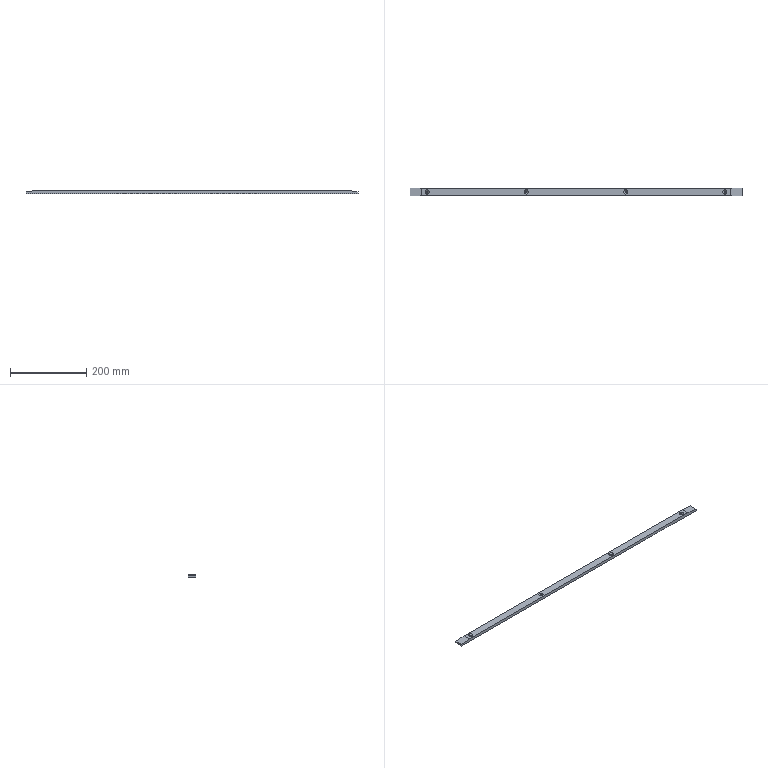Part | SolidWorks | features BaseBody 1 | 1 solid | 24 faces | box 870 x 20 x 8 mm | volume 136262 mm3 | cone 8 | cylinder 8 | plane 8 | commonest cylinder face diameters 5.5 x8
STEP:
#1=CARTESIAN_POINT('',(-392.75,0.,5.15));
#2=VERTEX_POINT('',#1);
#3=CARTESIAN_POINT('',(-387.25,0.,5.15));
#4=VERTEX_POINT('',#3);
#5=CARTESIAN_POINT('',(-390.,0.,5.15));
#6=DIRECTION('',(0.,0.,1.));
#7=DIRECTION('',(1.,0.,0.));
#8=AXIS2_PLACEMENT_3D('',#5,#6,#7);
#9=CIRCLE('',#8,2.75);
#10=EDGE_CURVE('',#2,#4,#9,.T.);
#11=ORIENTED_EDGE('',*,*,#10,.F.);
#12=CARTESIAN_POINT('',(-395.6,0.,8.));
#13=VERTEX_POINT('',#12);
#14=CARTESIAN_POINT('',(-395.6,0.,8.));
#15=DIRECTION('',(-0.7071,0.,0.7071));
#16=VECTOR('',#15,1000.);
#17=LINE('',#14,#16);
#18=EDGE_CURVE('',#2,#13,#17,.T.);
#19=ORIENTED_EDGE('',*,*,#18,.T.);
#20=CARTESIAN_POINT('',(-384.4,0.,8.));
#21=VERTEX_POINT('',#20);
#22=CARTESIAN_POINT('',(-390.,0.,8.));
#23=DIRECTION('',(0.,0.,1.));
#24=DIRECTION('',(1.,0.,0.));
#25=AXIS2_PLACEMENT_3D('',#22,#23,#24);
#26=CIRCLE('',#25,5.6);
#27=EDGE_CURVE('',#13,#21,#26,.T.);
#28=ORIENTED_EDGE('',*,*,#27,.T.);
#29=CARTESIAN_POINT('',(-384.4,0.,8.));
#30=DIRECTION('',(0.7071,0.,0.7071));
#31=VECTOR('',#30,1000.);
#32=LINE('',#29,#31);
#33=EDGE_CURVE('',#4,#21,#32,.T.);
#34=ORIENTED_EDGE('',*,*,#33,.F.);
#35=EDGE_LOOP('',(#11,#19,#28,#34));
#36=FACE_OUTER_BOUND('',#35,.T.);
#37=CARTESIAN_POINT('',(-390.,0.,8.));
#38=DIRECTION('',(0.,0.,1.));
#39=DIRECTION('',(1.,0.,0.));
#40=AXIS2_PLACEMENT_3D('',#37,#38,#39);
#41=CONICAL_SURFACE('',#40,5.6,0.7854);
#42=ADVANCED_FACE('',(#36),#41,.F.);
#43=CARTESIAN_POINT('',(-392.75,0.,0.));
#44=VERTEX_POINT('',#43);
#45=CARTESIAN_POINT('',(-387.25,0.,0.));
#46=VERTEX_POINT('',#45);
#47=CARTESIAN_POINT('',(-390.,0.,0.));
#48=DIRECTION('',(0.,0.,1.));
#49=DIRECTION('',(1.,0.,0.));
#50=AXIS2_PLACEMENT_3D('',#47,#48,#49);
#51=CIRCLE('',#50,2.75);
#52=EDGE_CURVE('',#44,#46,#51,.T.);
#53=ORIENTED_EDGE('',*,*,#52,.F.);
#54=CARTESIAN_POINT('',(-392.75,0.,8.));
#55=DIRECTION('',(0.,0.,1.));
#56=VECTOR('',#55,1000.);
#57=LINE('',#54,#56);
#58=EDGE_CURVE('',#44,#2,#57,.T.);
#59=ORIENTED_EDGE('',*,*,#58,.T.);
#60=ORIENTED_EDGE('',*,*,#10,.T.);
#61=CARTESIAN_POINT('',(-387.25,0.,8.));
#62=DIRECTION('',(0.,0.,1.));
#63=VECTOR('',#62,1000.);
#64=LINE('',#61,#63);
#65=EDGE_CURVE('',#46,#4,#64,.T.);
#66=ORIENTED_EDGE('',*,*,#65,.F.);
#67=EDGE_LOOP('',(#53,#59,#60,#66));
#68=FACE_OUTER_BOUND('',#67,.T.);
#69=CARTESIAN_POINT('',(-390.,0.,8.));
#70=DIRECTION('',(0.,0.,1.));
#71=DIRECTION('',(1.,0.,0.));
#72=AXIS2_PLACEMENT_3D('',#69,#70,#71);
#73=CYLINDRICAL_SURFACE('',#72,2.75);
#74=ADVANCED_FACE('',(#68),#73,.F.);
#75=CARTESIAN_POINT('',(-132.75,0.,5.15));
#76=VERTEX_POINT('',#75);
#77=CARTESIAN_POINT('',(-127.25,0.,5.15));
#78=VERTEX_POINT('',#77);
#79=CARTESIAN_POINT('',(-130.,0.,5.15));
#80=DIRECTION('',(0.,0.,1.));
#81=DIRECTION('',(1.,0.,0.));
#82=AXIS2_PLACEMENT_3D('',#79,#80,#81);
#83=CIRCLE('',#82,2.75);
#84=EDGE_CURVE('',#76,#78,#83,.T.);
#85=ORIENTED_EDGE('',*,*,#84,.F.);
#86=CARTESIAN_POINT('',(-135.6,0.,8.));
#87=VERTEX_POINT('',#86);
#88=CARTESIAN_POINT('',(-135.6,0.,8.));
#89=DIRECTION('',(-0.7071,0.,0.7071));
#90=VECTOR('',#89,1000.);
#91=LINE('',#88,#90);
#92=EDGE_CURVE('',#76,#87,#91,.T.);
#93=ORIENTED_EDGE('',*,*,#92,.T.);
#94=CARTESIAN_POINT('',(-124.4,0.,8.));
#95=VERTEX_POINT('',#94);
#96=CARTESIAN_POINT('',(-130.,0.,8.));
#97=DIRECTION('',(0.,0.,1.));
#98=DIRECTION('',(1.,0.,0.));
#99=AXIS2_PLACEMENT_3D('',#96,#97,#98);
#100=CIRCLE('',#99,5.6);
#101=EDGE_CURVE('',#87,#95,#100,.T.);
#102=ORIENTED_EDGE('',*,*,#101,.T.);
#103=CARTESIAN_POINT('',(-124.4,0.,8.));
#104=DIRECTION('',(0.7071,0.,0.7071));
#105=VECTOR('',#104,1000.);
#106=LINE('',#103,#105);
#107=EDGE_CURVE('',#78,#95,#106,.T.);
#108=ORIENTED_EDGE('',*,*,#107,.F.);
#109=EDGE_LOOP('',(#85,#93,#102,#108));
#110=FACE_OUTER_BOUND('',#109,.T.);
#111=CARTESIAN_POINT('',(-130.,0.,8.));
#112=DIRECTION('',(0.,0.,1.));
#113=DIRECTION('',(1.,0.,0.));
#114=AXIS2_PLACEMENT_3D('',#111,#112,#113);
#115=CONICAL_SURFACE('',#114,5.6,0.7854);
#116=ADVANCED_FACE('',(#110),#115,.F.);
#117=CARTESIAN_POINT('',(-132.75,0.,0.));
#118=VERTEX_POINT('',#117);
#119=CARTESIAN_POINT('',(-127.25,0.,0.));
#120=VERTEX_POINT('',#119);
#121=CARTESIAN_POINT('',(-130.,0.,0.));
#122=DIRECTION('',(0.,0.,1.));
#123=DIRECTION('',(1.,0.,0.));
#124=AXIS2_PLACEMENT_3D('',#121,#122,#123);
#125=CIRCLE('',#124,2.75);
#126=EDGE_CURVE('',#118,#120,#125,.T.);
#127=ORIENTED_EDGE('',*,*,#126,.F.);
#128=CARTESIAN_POINT('',(-132.75,0.,8.));
#129=DIRECTION('',(0.,0.,1.));
#130=VECTOR('',#129,1000.);
#131=LINE('',#128,#130);
#132=EDGE_CURVE('',#118,#76,#131,.T.);
#133=ORIENTED_EDGE('',*,*,#132,.T.);
#134=ORIENTED_EDGE('',*,*,#84,.T.);
#135=CARTESIAN_POINT('',(-127.25,0.,8.));
#136=DIRECTION('',(0.,0.,1.));
#137=VECTOR('',#136,1000.);
#138=LINE('',#135,#137);
#139=EDGE_CURVE('',#120,#78,#138,.T.);
#140=ORIENTED_EDGE('',*,*,#139,.F.);
#141=EDGE_LOOP('',(#127,#133,#134,#140));
#142=FACE_OUTER_BOUND('',#141,.T.);
#143=CARTESIAN_POINT('',(-130.,0.,8.));
#144=DIRECTION('',(0.,0.,1.));
#145=DIRECTION('',(1.,0.,0.));
#146=AXIS2_PLACEMENT_3D('',#143,#144,#145);
#147=CYLINDRICAL_SURFACE('',#146,2.75);
#148=ADVANCED_FACE('',(#142),#147,.F.);
#149=CARTESIAN_POINT('',(127.25,0.,5.15));
#150=VERTEX_POINT('',#149);
#151=CARTESIAN_POINT('',(132.75,0.,5.15));
#152=VERTEX_POINT('',#151);
#153=CARTESIAN_POINT('',(130.,0.,5.15));
#154=DIRECTION('',(0.,0.,1.));
#155=DIRECTION('',(1.,0.,0.));
#156=AXIS2_PLACEMENT_3D('',#153,#154,#155);
#157=CIRCLE('',#156,2.75);
#158=EDGE_CURVE('',#150,#152,#157,.T.);
#159=ORIENTED_EDGE('',*,*,#158,.F.);
#160=CARTESIAN_POINT('',(124.4,0.,8.));
#161=VERTEX_POINT('',#160);
#162=CARTESIAN_POINT('',(124.4,0.,8.));
#163=DIRECTION('',(-0.7071,0.,0.7071));
#164=VECTOR('',#163,1000.);
#165=LINE('',#162,#164);
#166=EDGE_CURVE('',#150,#161,#165,.T.);
#167=ORIENTED_EDGE('',*,*,#166,.T.);
#168=CARTESIAN_POINT('',(135.6,0.,8.));
#169=VERTEX_POINT('',#168);
#170=CARTESIAN_POINT('',(130.,0.,8.));
#171=DIRECTION('',(0.,0.,1.));
#172=DIRECTION('',(1.,0.,0.));
#173=AXIS2_PLACEMENT_3D('',#170,#171,#172);
#174=CIRCLE('',#173,5.6);
#175=EDGE_CURVE('',#161,#169,#174,.T.);
#176=ORIENTED_EDGE('',*,*,#175,.T.);
#177=CARTESIAN_POINT('',(135.6,0.,8.));
#178=DIRECTION('',(0.7071,0.,0.7071));
#179=VECTOR('',#178,1000.);
#180=LINE('',#177,#179);
#181=EDGE_CURVE('',#152,#169,#180,.T.);
#182=ORIENTED_EDGE('',*,*,#181,.F.);
#183=EDGE_LOOP('',(#159,#167,#176,#182));
#184=FACE_OUTER_BOUND('',#183,.T.);
#185=CARTESIAN_POINT('',(130.,0.,8.));
#186=DIRECTION('',(0.,0.,1.));
#187=DIRECTION('',(1.,0.,0.));
#188=AXIS2_PLACEMENT_3D('',#185,#186,#187);
#189=CONICAL_SURFACE('',#188,5.6,0.7854);
#190=ADVANCED_FACE('',(#184),#189,.F.);
#191=CARTESIAN_POINT('',(127.25,0.,0.));
#192=VERTEX_POINT('',#191);
#193=CARTESIAN_POINT('',(132.75,0.,0.));
#194=VERTEX_POINT('',#193);
#195=CARTESIAN_POINT('',(130.,0.,0.));
#196=DIRECTION('',(0.,0.,1.));
#197=DIRECTION('',(1.,0.,0.));
#198=AXIS2_PLACEMENT_3D('',#195,#196,#197);
#199=CIRCLE('',#198,2.75);
#200=EDGE_CURVE('',#192,#194,#199,.T.);
#201=ORIENTED_EDGE('',*,*,#200,.F.);
#202=CARTESIAN_POINT('',(127.25,0.,8.));
#203=DIRECTION('',(0.,0.,1.));
#204=VECTOR('',#203,1000.);
#205=LINE('',#202,#204);
#206=EDGE_CURVE('',#192,#150,#205,.T.);
#207=ORIENTED_EDGE('',*,*,#206,.T.);
#208=ORIENTED_EDGE('',*,*,#158,.T.);
#209=CARTESIAN_POINT('',(132.75,0.,8.));
#210=DIRECTION('',(0.,0.,1.));
#211=VECTOR('',#210,1000.);
#212=LINE('',#209,#211);
#213=EDGE_CURVE('',#194,#152,#212,.T.);
#214=ORIENTED_EDGE('',*,*,#213,.F.);
#215=EDGE_LOOP('',(#201,#207,#208,#214));
#216=FACE_OUTER_BOUND('',#215,.T.);
#217=CARTESIAN_POINT('',(130.,0.,8.));
#218=DIRECTION('',(0.,0.,1.));
#219=DIRECTION('',(1.,0.,0.));
#220=AXIS2_PLACEMENT_3D('',#217,#218,#219);
#221=CYLINDRICAL_SURFACE('',#220,2.75);
#222=ADVANCED_FACE('',(#216),#221,.F.);
#223=CARTESIAN_POINT('',(387.25,0.,5.15));
#224=VERTEX_POINT('',#223);
#225=CARTESIAN_POINT('',(392.75,0.,5.15));
#226=VERTEX_POINT('',#225);
#227=CARTESIAN_POINT('',(390.,0.,5.15));
#228=DIRECTION('',(0.,0.,1.));
#229=DIRECTION('',(1.,0.,0.));
#230=AXIS2_PLACEMENT_3D('',#227,#228,#229);
#231=CIRCLE('',#230,2.75);
#232=EDGE_CURVE('',#224,#226,#231,.T.);
#233=ORIENTED_EDGE('',*,*,#232,.F.);
#234=CARTESIAN_POINT('',(384.4,0.,8.));
#235=VERTEX_POINT('',#234);
#236=CARTESIAN_POINT('',(384.4,0.,8.));
#237=DIRECTION('',(-0.7071,0.,0.7071));
#238=VECTOR('',#237,1000.);
#239=LINE('',#236,#238);
#240=EDGE_CURVE('',#224,#235,#239,.T.);
#241=ORIENTED_EDGE('',*,*,#240,.T.);
#242=CARTESIAN_POINT('',(395.6,0.,8.));
#243=VERTEX_POINT('',#242);
#244=CARTESIAN_POINT('',(390.,0.,8.));
#245=DIRECTION('',(0.,0.,1.));
#246=DIRECTION('',(1.,0.,0.));
#247=AXIS2_PLACEMENT_3D('',#244,#245,#246);
#248=CIRCLE('',#247,5.6);
#249=EDGE_CURVE('',#235,#243,#248,.T.);
#250=ORIENTED_EDGE('',*,*,#249,.T.);
#251=CARTESIAN_POINT('',(395.6,0.,8.));
#252=DIRECTION('',(0.7071,0.,0.7071));
#253=VECTOR('',#252,1000.);
#254=LINE('',#251,#253);
#255=EDGE_CURVE('',#226,#243,#254,.T.);
#256=ORIENTED_EDGE('',*,*,#255,.F.);
#257=EDGE_LOOP('',(#233,#241,#250,#256));
#258=FACE_OUTER_BOUND('',#257,.T.);
#259=CARTESIAN_POINT('',(390.,0.,8.));
#260=DIRECTION('',(0.,0.,1.));
#261=DIRECTION('',(1.,0.,0.));
#262=AXIS2_PLACEMENT_3D('',#259,#260,#261);
#263=CONICAL_SURFACE('',#262,5.6,0.7854);
#264=ADVANCED_FACE('',(#258),#263,.F.);
#265=CARTESIAN_POINT('',(387.25,0.,0.));
#266=VERTEX_POINT('',#265);
#267=CARTESIAN_POINT('',(392.75,0.,0.));
#268=VERTEX_POINT('',#267);
#269=CARTESIAN_POINT('',(390.,0.,0.));
#270=DIRECTION('',(0.,0.,1.));
#271=DIRECTION('',(1.,0.,0.));
#272=AXIS2_PLACEMENT_3D('',#269,#270,#271);
#273=CIRCLE('',#272,2.75);
#274=EDGE_CURVE('',#266,#268,#273,.T.);
#275=ORIENTED_EDGE('',*,*,#274,.F.);
#276=CARTESIAN_POINT('',(387.25,0.,8.));
#277=DIRECTION('',(0.,0.,1.));
#278=VECTOR('',#277,1000.);
#279=LINE('',#276,#278);
#280=EDGE_CURVE('',#266,#224,#279,.T.);
#281=ORIENTED_EDGE('',*,*,#280,.T.);
#282=ORIENTED_EDGE('',*,*,#232,.T.);
#283=CARTESIAN_POINT('',(392.75,0.,8.));
#284=DIRECTION('',(0.,0.,1.));
#285=VECTOR('',#284,1000.);
#286=LINE('',#283,#285);
#287=EDGE_CURVE('',#268,#226,#286,.T.);
#288=ORIENTED_EDGE('',*,*,#287,.F.);
#289=EDGE_LOOP('',(#275,#281,#282,#288));
#290=FACE_OUTER_BOUND('',#289,.T.);
#291=CARTESIAN_POINT('',(390.,0.,8.));
#292=DIRECTION('',(0.,0.,1.));
#293=DIRECTION('',(1.,0.,0.));
#294=AXIS2_PLACEMENT_3D('',#291,#292,#293);
#295=CYLINDRICAL_SURFACE('',#294,2.75);
#296=ADVANCED_FACE('',(#290),#295,.F.);
#297=CARTESIAN_POINT('',(435.,10.,5.));
#298=VERTEX_POINT('',#297);
#299=CARTESIAN_POINT('',(435.,10.,0.));
#300=VERTEX_POINT('',#299);
#301=CARTESIAN_POINT('',(435.,10.,8.));
#302=DIRECTION('',(0.,0.,-1.));
#303=VECTOR('',#302,1000.);
#304=LINE('',#301,#303);
#305=EDGE_CURVE('',#298,#300,#304,.T.);
#306=ORIENTED_EDGE('',*,*,#305,.F.);
#307=CARTESIAN_POINT('',(435.,-10.,5.));
#308=VERTEX_POINT('',#307);
#309=CARTESIAN_POINT('',(435.,-10.,5.));
#310=DIRECTION('',(0.,-1.,0.));
#311=VECTOR('',#310,1000.);
#312=LINE('',#309,#311);
#313=EDGE_CURVE('',#298,#308,#312,.T.);
#314=ORIENTED_EDGE('',*,*,#313,.T.);
#315=CARTESIAN_POINT('',(435.,-10.,0.));
#316=VERTEX_POINT('',#315);
#317=CARTESIAN_POINT('',(435.,-10.,8.));
#318=DIRECTION('',(0.,0.,-1.));
#319=VECTOR('',#318,1000.);
#320=LINE('',#317,#319);
#321=EDGE_CURVE('',#308,#316,#320,.T.);
#322=ORIENTED_EDGE('',*,*,#321,.T.);
#323=CARTESIAN_POINT('',(435.,10.,0.));
#324=DIRECTION('',(0.,1.,0.));
#325=VECTOR('',#324,1000.);
#326=LINE('',#323,#325);
#327=EDGE_CURVE('',#316,#300,#326,.T.);
#328=ORIENTED_EDGE('',*,*,#327,.T.);
#329=EDGE_LOOP('',(#306,#314,#322,#328));
#330=FACE_OUTER_BOUND('',#329,.T.);
#331=CARTESIAN_POINT('',(435.,10.,8.));
#332=DIRECTION('',(-1.,0.,0.));
#333=DIRECTION('',(0.,0.,1.));
#334=AXIS2_PLACEMENT_3D('',#331,#332,#333);
#335=PLANE('',#334);
#336=ADVANCED_FACE('',(#330),#335,.F.);
#337=CARTESIAN_POINT('',(405.,10.,8.));
#338=VERTEX_POINT('',#337);
#339=CARTESIAN_POINT('',(-405.,10.,8.));
#340=VERTEX_POINT('',#339);
#341=CARTESIAN_POINT('',(-435.,10.,8.));
#342=DIRECTION('',(-1.,0.,0.));
#343=VECTOR('',#342,1000.);
#344=LINE('',#341,#343);
#345=EDGE_CURVE('',#338,#340,#344,.T.);
#346=ORIENTED_EDGE('',*,*,#345,.F.);
#347=CARTESIAN_POINT('',(405.,10.,8.));
#348=DIRECTION('',(0.995,0.,-0.0995));
#349=VECTOR('',#348,1000.);
#350=LINE('',#347,#349);
#351=EDGE_CURVE('',#338,#298,#350,.T.);
#352=ORIENTED_EDGE('',*,*,#351,.T.);
#353=ORIENTED_EDGE('',*,*,#305,.T.);
#354=CARTESIAN_POINT('',(-435.,10.,0.));
#355=VERTEX_POINT('',#354);
#356=CARTESIAN_POINT('',(-435.,10.,0.));
#357=DIRECTION('',(-1.,0.,0.));
#358=VECTOR('',#357,1000.);
#359=LINE('',#356,#358);
#360=EDGE_CURVE('',#300,#355,#359,.T.);
#361=ORIENTED_EDGE('',*,*,#360,.T.);
#362=CARTESIAN_POINT('',(-435.,10.,5.));
#363=VERTEX_POINT('',#362);
#364=CARTESIAN_POINT('',(-435.,10.,8.));
#365=DIRECTION('',(0.,0.,-1.));
#366=VECTOR('',#365,1000.);
#367=LINE('',#364,#366);
#368=EDGE_CURVE('',#363,#355,#367,.T.);
#369=ORIENTED_EDGE('',*,*,#368,.F.);
#370=CARTESIAN_POINT('',(-405.,10.,8.));
#371=DIRECTION('',(0.995,0.,0.0995));
#372=VECTOR('',#371,1000.);
#373=LINE('',#370,#372);
#374=EDGE_CURVE('',#363,#340,#373,.T.);
#375=ORIENTED_EDGE('',*,*,#374,.T.);
#376=EDGE_LOOP('',(#346,#352,#353,#361,#369,#375));
#377=FACE_OUTER_BOUND('',#376,.T.);
#378=CARTESIAN_POINT('',(-435.,10.,8.));
#379=DIRECTION('',(0.,-1.,0.));
#380=DIRECTION('',(0.,0.,-1.));
#381=AXIS2_PLACEMENT_3D('',#378,#379,#380);
#382=PLANE('',#381);
#383=ADVANCED_FACE('',(#377),#382,.F.);
#384=CARTESIAN_POINT('',(-435.,-10.,5.));
#385=VERTEX_POINT('',#384);
#386=CARTESIAN_POINT('',(-435.,-10.,0.));
#387=VERTEX_POINT('',#386);
#388=CARTESIAN_POINT('',(-435.,-10.,8.));
#389=DIRECTION('',(0.,0.,-1.));
#390=VECTOR('',#389,1000.);
#391=LINE('',#388,#390);
#392=EDGE_CURVE('',#385,#387,#391,.T.);
#393=ORIENTED_EDGE('',*,*,#392,.F.);
#394=CARTESIAN_POINT('',(-435.,10.,5.));
#395=DIRECTION('',(0.,1.,0.));
#396=VECTOR('',#395,1000.);
#397=LINE('',#394,#396);
#398=EDGE_CURVE('',#385,#363,#397,.T.);
#399=ORIENTED_EDGE('',*,*,#398,.T.);
#400=ORIENTED_EDGE('',*,*,#368,.T.);
#401=CARTESIAN_POINT('',(-435.,10.,0.));
#402=DIRECTION('',(0.,-1.,0.));
#403=VECTOR('',#402,1000.);
#404=LINE('',#401,#403);
#405=EDGE_CURVE('',#355,#387,#404,.T.);
#406=ORIENTED_EDGE('',*,*,#405,.T.);
#407=EDGE_LOOP('',(#393,#399,#400,#406));
#408=FACE_OUTER_BOUND('',#407,.T.);
#409=CARTESIAN_POINT('',(-435.,10.,8.));
#410=DIRECTION('',(1.,0.,0.));
#411=DIRECTION('',(0.,0.,-1.));
#412=AXIS2_PLACEMENT_3D('',#409,#410,#411);
#413=PLANE('',#412);
#414=ADVANCED_FACE('',(#408),#413,.F.);
#415=ORIENTED_EDGE('',*,*,#321,.F.);
#416=CARTESIAN_POINT('',(405.,-10.,8.));
#417=VERTEX_POINT('',#416);
#418=CARTESIAN_POINT('',(405.,-10.,8.));
#419=DIRECTION('',(-0.995,0.,0.0995));
#420=VECTOR('',#419,1000.);
#421=LINE('',#418,#420);
#422=EDGE_CURVE('',#308,#417,#421,.T.);
#423=ORIENTED_EDGE('',*,*,#422,.T.);
#424=CARTESIAN_POINT('',(-405.,-10.,8.));
#425=VERTEX_POINT('',#424);
#426=CARTESIAN_POINT('',(-435.,-10.,8.));
#427=DIRECTION('',(1.,0.,0.));
#428=VECTOR('',#427,1000.);
#429=LINE('',#426,#428);
#430=EDGE_CURVE('',#425,#417,#429,.T.);
#431=ORIENTED_EDGE('',*,*,#430,.F.);
#432=CARTESIAN_POINT('',(-405.,-10.,8.));
#433=DIRECTION('',(-0.995,0.,-0.0995));
#434=VECTOR('',#433,1000.);
#435=LINE('',#432,#434);
#436=EDGE_CURVE('',#425,#385,#435,.T.);
#437=ORIENTED_EDGE('',*,*,#436,.T.);
#438=ORIENTED_EDGE('',*,*,#392,.T.);
#439=CARTESIAN_POINT('',(-435.,-10.,0.));
#440=DIRECTION('',(1.,0.,0.));
#441=VECTOR('',#440,1000.);
#442=LINE('',#439,#441);
#443=EDGE_CURVE('',#387,#316,#442,.T.);
#444=ORIENTED_EDGE('',*,*,#443,.T.);
#445=EDGE_LOOP('',(#415,#423,#431,#437,#438,#444));
#446=FACE_OUTER_BOUND('',#445,.T.);
#447=CARTESIAN_POINT('',(-435.,-10.,8.));
#448=DIRECTION('',(0.,1.,0.));
#449=DIRECTION('',(0.,0.,1.));
#450=AXIS2_PLACEMENT_3D('',#447,#448,#449);
#451=PLANE('',#450);
#452=ADVANCED_FACE('',(#446),#451,.F.);
#453=CARTESIAN_POINT('',(-390.,0.,8.));
#454=DIRECTION('',(0.,0.,1.));
#455=DIRECTION('',(1.,0.,0.));
#456=AXIS2_PLACEMENT_3D('',#453,#454,#455);
#457=CIRCLE('',#456,5.6);
#458=EDGE_CURVE('',#21,#13,#457,.T.);
#459=ORIENTED_EDGE('',*,*,#458,.F.);
#460=ORIENTED_EDGE('',*,*,#27,.F.);
#461=EDGE_LOOP('',(#459,#460));
#462=FACE_BOUND('',#461,.T.);
#463=CARTESIAN_POINT('',(-130.,0.,8.));
#464=DIRECTION('',(0.,0.,1.));
#465=DIRECTION('',(1.,0.,0.));
#466=AXIS2_PLACEMENT_3D('',#463,#464,#465);
#467=CIRCLE('',#466,5.6);
#468=EDGE_CURVE('',#95,#87,#467,.T.);
#469=ORIENTED_EDGE('',*,*,#468,.F.);
#470=ORIENTED_EDGE('',*,*,#101,.F.);
#471=EDGE_LOOP('',(#469,#470));
#472=FACE_BOUND('',#471,.T.);
#473=CARTESIAN_POINT('',(130.,0.,8.));
#474=DIRECTION('',(0.,0.,1.));
#475=DIRECTION('',(1.,0.,0.));
#476=AXIS2_PLACEMENT_3D('',#473,#474,#475);
#477=CIRCLE('',#476,5.6);
#478=EDGE_CURVE('',#169,#161,#477,.T.);
#479=ORIENTED_EDGE('',*,*,#478,.F.);
#480=ORIENTED_EDGE('',*,*,#175,.F.);
#481=EDGE_LOOP('',(#479,#480));
#482=FACE_BOUND('',#481,.T.);
#483=CARTESIAN_POINT('',(390.,0.,8.));
#484=DIRECTION('',(0.,0.,1.));
#485=DIRECTION('',(1.,0.,0.));
#486=AXIS2_PLACEMENT_3D('',#483,#484,#485);
#487=CIRCLE('',#486,5.6);
#488=EDGE_CURVE('',#243,#235,#487,.T.);
#489=ORIENTED_EDGE('',*,*,#488,.F.);
#490=ORIENTED_EDGE('',*,*,#249,.F.);
#491=EDGE_LOOP('',(#489,#490));
#492=FACE_BOUND('',#491,.T.);
#493=ORIENTED_EDGE('',*,*,#430,.T.);
#494=CARTESIAN_POINT('',(405.,10.,8.));
#495=DIRECTION('',(0.,1.,0.));
#496=VECTOR('',#495,1000.);
#497=LINE('',#494,#496);
#498=EDGE_CURVE('',#417,#338,#497,.T.);
#499=ORIENTED_EDGE('',*,*,#498,.T.);
#500=ORIENTED_EDGE('',*,*,#345,.T.);
#501=CARTESIAN_POINT('',(-405.,-10.,8.));
#502=DIRECTION('',(0.,-1.,0.));
#503=VECTOR('',#502,1000.);
#504=LINE('',#501,#503);
#505=EDGE_CURVE('',#340,#425,#504,.T.);
#506=ORIENTED_EDGE('',*,*,#505,.T.);
#507=EDGE_LOOP('',(#493,#499,#500,#506));
#508=FACE_OUTER_BOUND('',#507,.T.);
#509=CARTESIAN_POINT('',(0.,0.,8.));
#510=DIRECTION('',(0.,0.,1.));
#511=DIRECTION('',(1.,0.,0.));
#512=AXIS2_PLACEMENT_3D('',#509,#510,#511);
#513=PLANE('',#512);
#514=ADVANCED_FACE('',(#462,#472,#482,#492,#508),#513,.T.);
#515=CARTESIAN_POINT('',(-390.,0.,0.));
#516=DIRECTION('',(0.,0.,1.));
#517=DIRECTION('',(1.,0.,0.));
#518=AXIS2_PLACEMENT_3D('',#515,#516,#517);
#519=CIRCLE('',#518,2.75);
#520=EDGE_CURVE('',#46,#44,#519,.T.);
#521=ORIENTED_EDGE('',*,*,#520,.T.);
#522=ORIENTED_EDGE('',*,*,#52,.T.);
#523=EDGE_LOOP('',(#521,#522));
#524=FACE_BOUND('',#523,.T.);
#525=CARTESIAN_POINT('',(-130.,0.,0.));
#526=DIRECTION('',(0.,0.,1.));
#527=DIRECTION('',(1.,0.,0.));
#528=AXIS2_PLACEMENT_3D('',#525,#526,#527);
#529=CIRCLE('',#528,2.75);
#530=EDGE_CURVE('',#120,#118,#529,.T.);
#531=ORIENTED_EDGE('',*,*,#530,.T.);
#532=ORIENTED_EDGE('',*,*,#126,.T.);
#533=EDGE_LOOP('',(#531,#532));
#534=FACE_BOUND('',#533,.T.);
#535=CARTESIAN_POINT('',(130.,0.,0.));
#536=DIRECTION('',(0.,0.,1.));
#537=DIRECTION('',(1.,0.,0.));
#538=AXIS2_PLACEMENT_3D('',#535,#536,#537);
#539=CIRCLE('',#538,2.75);
#540=EDGE_CURVE('',#194,#192,#539,.T.);
#541=ORIENTED_EDGE('',*,*,#540,.T.);
#542=ORIENTED_EDGE('',*,*,#200,.T.);
#543=EDGE_LOOP('',(#541,#542));
#544=FACE_BOUND('',#543,.T.);
#545=CARTESIAN_POINT('',(390.,0.,0.));
#546=DIRECTION('',(0.,0.,1.));
#547=DIRECTION('',(1.,0.,0.));
#548=AXIS2_PLACEMENT_3D('',#545,#546,#547);
#549=CIRCLE('',#548,2.75);
#550=EDGE_CURVE('',#268,#266,#549,.T.);
#551=ORIENTED_EDGE('',*,*,#550,.T.);
#552=ORIENTED_EDGE('',*,*,#274,.T.);
#553=EDGE_LOOP('',(#551,#552));
#554=FACE_BOUND('',#553,.T.);
#555=ORIENTED_EDGE('',*,*,#327,.F.);
#556=ORIENTED_EDGE('',*,*,#443,.F.);
#557=ORIENTED_EDGE('',*,*,#405,.F.);
#558=ORIENTED_EDGE('',*,*,#360,.F.);
#559=EDGE_LOOP('',(#555,#556,#557,#558));
#560=FACE_OUTER_BOUND('',#559,.T.);
#561=CARTESIAN_POINT('',(0.,0.,0.));
#562=DIRECTION('',(0.,0.,1.));
#563=DIRECTION('',(1.,0.,0.));
#564=AXIS2_PLACEMENT_3D('',#561,#562,#563);
#565=PLANE('',#564);
#566=ADVANCED_FACE('',(#524,#534,#544,#554,#560),#565,.F.);
#567=ORIENTED_EDGE('',*,*,#374,.F.);
#568=ORIENTED_EDGE('',*,*,#398,.F.);
#569=ORIENTED_EDGE('',*,*,#436,.F.);
#570=ORIENTED_EDGE('',*,*,#505,.F.);
#571=EDGE_LOOP('',(#567,#568,#569,#570));
#572=FACE_OUTER_BOUND('',#571,.T.);
#573=CARTESIAN_POINT('',(-405.,0.,8.));
#574=DIRECTION('',(-0.0995,0.,0.995));
#575=DIRECTION('',(0.,1.,0.));
#576=AXIS2_PLACEMENT_3D('',#573,#574,#575);
#577=PLANE('',#576);
#578=ADVANCED_FACE('',(#572),#577,.T.);
#579=ORIENTED_EDGE('',*,*,#422,.F.);
#580=ORIENTED_EDGE('',*,*,#313,.F.);
#581=ORIENTED_EDGE('',*,*,#351,.F.);
#582=ORIENTED_EDGE('',*,*,#498,.F.);
#583=EDGE_LOOP('',(#579,#580,#581,#582));
#584=FACE_OUTER_BOUND('',#583,.T.);
#585=CARTESIAN_POINT('',(405.,0.,8.));
#586=DIRECTION('',(0.0995,0.,0.995));
#587=DIRECTION('',(0.,-1.,0.));
#588=AXIS2_PLACEMENT_3D('',#585,#586,#587);
#589=PLANE('',#588);
#590=ADVANCED_FACE('',(#584),#589,.T.);
#591=ORIENTED_EDGE('',*,*,#280,.F.);
#592=ORIENTED_EDGE('',*,*,#550,.F.);
#593=ORIENTED_EDGE('',*,*,#287,.T.);
#594=CARTESIAN_POINT('',(390.,0.,5.15));
#595=DIRECTION('',(0.,0.,1.));
#596=DIRECTION('',(1.,0.,0.));
#597=AXIS2_PLACEMENT_3D('',#594,#595,#596);
#598=CIRCLE('',#597,2.75);
#599=EDGE_CURVE('',#226,#224,#598,.T.);
#600=ORIENTED_EDGE('',*,*,#599,.T.);
#601=EDGE_LOOP('',(#591,#592,#593,#600));
#602=FACE_OUTER_BOUND('',#601,.T.);
#603=CARTESIAN_POINT('',(390.,0.,8.));
#604=DIRECTION('',(0.,0.,1.));
#605=DIRECTION('',(1.,0.,0.));
#606=AXIS2_PLACEMENT_3D('',#603,#604,#605);
#607=CYLINDRICAL_SURFACE('',#606,2.75);
#608=ADVANCED_FACE('',(#602),#607,.F.);
#609=ORIENTED_EDGE('',*,*,#240,.F.);
#610=ORIENTED_EDGE('',*,*,#599,.F.);
#611=ORIENTED_EDGE('',*,*,#255,.T.);
#612=ORIENTED_EDGE('',*,*,#488,.T.);
#613=EDGE_LOOP('',(#609,#610,#611,#612));
#614=FACE_OUTER_BOUND('',#613,.T.);
#615=CARTESIAN_POINT('',(390.,0.,8.));
#616=DIRECTION('',(0.,0.,1.));
#617=DIRECTION('',(1.,0.,0.));
#618=AXIS2_PLACEMENT_3D('',#615,#616,#617);
#619=CONICAL_SURFACE('',#618,5.6,0.7854);
#620=ADVANCED_FACE('',(#614),#619,.F.);
#621=ORIENTED_EDGE('',*,*,#206,.F.);
#622=ORIENTED_EDGE('',*,*,#540,.F.);
#623=ORIENTED_EDGE('',*,*,#213,.T.);
#624=CARTESIAN_POINT('',(130.,0.,5.15));
#625=DIRECTION('',(0.,0.,1.));
#626=DIRECTION('',(1.,0.,0.));
#627=AXIS2_PLACEMENT_3D('',#624,#625,#626);
#628=CIRCLE('',#627,2.75);
#629=EDGE_CURVE('',#152,#150,#628,.T.);
#630=ORIENTED_EDGE('',*,*,#629,.T.);
#631=EDGE_LOOP('',(#621,#622,#623,#630));
#632=FACE_OUTER_BOUND('',#631,.T.);
#633=CARTESIAN_POINT('',(130.,0.,8.));
#634=DIRECTION('',(0.,0.,1.));
#635=DIRECTION('',(1.,0.,0.));
#636=AXIS2_PLACEMENT_3D('',#633,#634,#635);
#637=CYLINDRICAL_SURFACE('',#636,2.75);
#638=ADVANCED_FACE('',(#632),#637,.F.);
#639=ORIENTED_EDGE('',*,*,#166,.F.);
#640=ORIENTED_EDGE('',*,*,#629,.F.);
#641=ORIENTED_EDGE('',*,*,#181,.T.);
#642=ORIENTED_EDGE('',*,*,#478,.T.);
#643=EDGE_LOOP('',(#639,#640,#641,#642));
#644=FACE_OUTER_BOUND('',#643,.T.);
#645=CARTESIAN_POINT('',(130.,0.,8.));
#646=DIRECTION('',(0.,0.,1.));
#647=DIRECTION('',(1.,0.,0.));
#648=AXIS2_PLACEMENT_3D('',#645,#646,#647);
#649=CONICAL_SURFACE('',#648,5.6,0.7854);
#650=ADVANCED_FACE('',(#644),#649,.F.);
#651=ORIENTED_EDGE('',*,*,#132,.F.);
#652=ORIENTED_EDGE('',*,*,#530,.F.);
#653=ORIENTED_EDGE('',*,*,#139,.T.);
#654=CARTESIAN_POINT('',(-130.,0.,5.15));
#655=DIRECTION('',(0.,0.,1.));
#656=DIRECTION('',(1.,0.,0.));
#657=AXIS2_PLACEMENT_3D('',#654,#655,#656);
#658=CIRCLE('',#657,2.75);
#659=EDGE_CURVE('',#78,#76,#658,.T.);
#660=ORIENTED_EDGE('',*,*,#659,.T.);
#661=EDGE_LOOP('',(#651,#652,#653,#660));
#662=FACE_OUTER_BOUND('',#661,.T.);
#663=CARTESIAN_POINT('',(-130.,0.,8.));
#664=DIRECTION('',(0.,0.,1.));
#665=DIRECTION('',(1.,0.,0.));
#666=AXIS2_PLACEMENT_3D('',#663,#664,#665);
#667=CYLINDRICAL_SURFACE('',#666,2.75);
#668=ADVANCED_FACE('',(#662),#667,.F.);
#669=ORIENTED_EDGE('',*,*,#92,.F.);
#670=ORIENTED_EDGE('',*,*,#659,.F.);
#671=ORIENTED_EDGE('',*,*,#107,.T.);
#672=ORIENTED_EDGE('',*,*,#468,.T.);
#673=EDGE_LOOP('',(#669,#670,#671,#672));
#674=FACE_OUTER_BOUND('',#673,.T.);
#675=CARTESIAN_POINT('',(-130.,0.,8.));
#676=DIRECTION('',(0.,0.,1.));
#677=DIRECTION('',(1.,0.,0.));
#678=AXIS2_PLACEMENT_3D('',#675,#676,#677);
#679=CONICAL_SURFACE('',#678,5.6,0.7854);
#680=ADVANCED_FACE('',(#674),#679,.F.);
#681=ORIENTED_EDGE('',*,*,#58,.F.);
#682=ORIENTED_EDGE('',*,*,#520,.F.);
#683=ORIENTED_EDGE('',*,*,#65,.T.);
#684=CARTESIAN_POINT('',(-390.,0.,5.15));
#685=DIRECTION('',(0.,0.,1.));
#686=DIRECTION('',(1.,0.,0.));
#687=AXIS2_PLACEMENT_3D('',#684,#685,#686);
#688=CIRCLE('',#687,2.75);
#689=EDGE_CURVE('',#4,#2,#688,.T.);
#690=ORIENTED_EDGE('',*,*,#689,.T.);
#691=EDGE_LOOP('',(#681,#682,#683,#690));
#692=FACE_OUTER_BOUND('',#691,.T.);
#693=CARTESIAN_POINT('',(-390.,0.,8.));
#694=DIRECTION('',(0.,0.,1.));
#695=DIRECTION('',(1.,0.,0.));
#696=AXIS2_PLACEMENT_3D('',#693,#694,#695);
#697=CYLINDRICAL_SURFACE('',#696,2.75);
#698=ADVANCED_FACE('',(#692),#697,.F.);
#699=ORIENTED_EDGE('',*,*,#18,.F.);
#700=ORIENTED_EDGE('',*,*,#689,.F.);
#701=ORIENTED_EDGE('',*,*,#33,.T.);
#702=ORIENTED_EDGE('',*,*,#458,.T.);
#703=EDGE_LOOP('',(#699,#700,#701,#702));
#704=FACE_OUTER_BOUND('',#703,.T.);
#705=CARTESIAN_POINT('',(-390.,0.,8.));
#706=DIRECTION('',(0.,0.,1.));
#707=DIRECTION('',(1.,0.,0.));
#708=AXIS2_PLACEMENT_3D('',#705,#706,#707);
#709=CONICAL_SURFACE('',#708,5.6,0.7854);
#710=ADVANCED_FACE('',(#704),#709,.F.);
#711=CLOSED_SHELL('',(#42,#74,#116,#148,#190,#222,#264,#296,#336,#383,#414,#452,#514,#566,#578,#590,#608,#620,#638,#650,#668,#680,#698,#710));
#712=MANIFOLD_SOLID_BREP('',#711);
#713=CARTESIAN_POINT('',(0.,0.,0.));
#714=DIRECTION('',(0.,0.,1.));
#715=DIRECTION('',(1.,0.,0.));
#716=AXIS2_PLACEMENT_3D('',#713,#714,#715);
#717=(LENGTH_UNIT()NAMED_UNIT(*)SI_UNIT(.MILLI.,.METRE.));
#718=UNCERTAINTY_MEASURE_WITH_UNIT(LENGTH_MEASURE(0.00001),#717,'','');
#719=(NAMED_UNIT(*)PLANE_ANGLE_UNIT()SI_UNIT($,.RADIAN.));
#720=(NAMED_UNIT(*)SI_UNIT($,.STERADIAN.)SOLID_ANGLE_UNIT());
#721=(GEOMETRIC_REPRESENTATION_CONTEXT(3)GLOBAL_UNCERTAINTY_ASSIGNED_CONTEXT((#718))GLOBAL_UNIT_ASSIGNED_CONTEXT((#717,#719,#720))REPRESENTATION_CONTEXT('',''));
#722=ADVANCED_BREP_SHAPE_REPRESENTATION('',(#712,#716),#721);